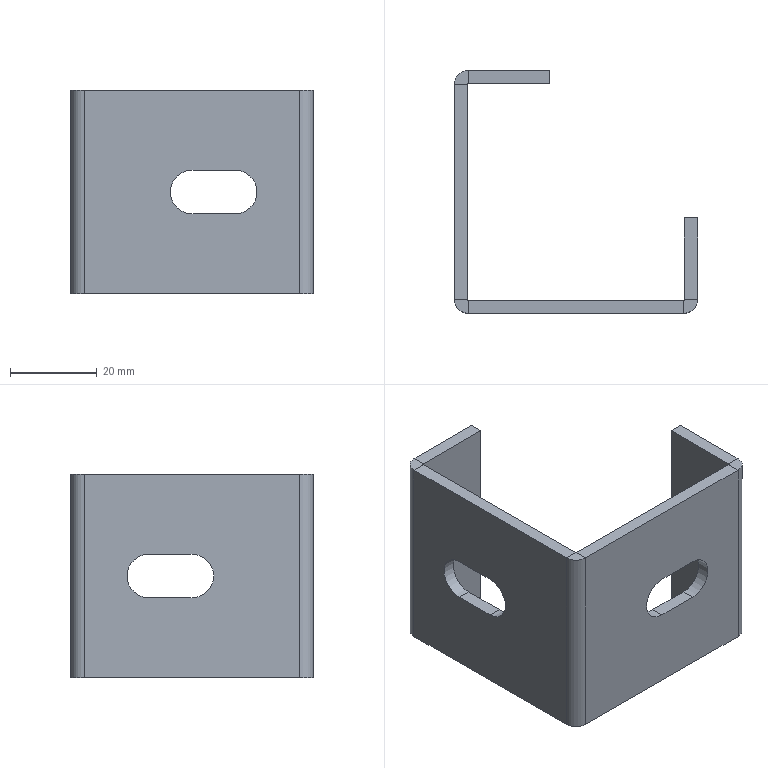Part | SolidWorks | features ICE 3, FlatPattern 1, SMBaseFlange 1, SheetMetal 1 | 1 solid | 39 faces | box 56 x 56 x 47 mm | volume 19347 mm3 | plane 28 | cylinder 11 | commonest cylinder face diameters 10 x5 0.4 x3 6.4 x3
STEP:
#1=CARTESIAN_POINT('',(3.,23.,0.));
#2=VERTEX_POINT('',#1);
#3=CARTESIAN_POINT('',(3.,28.,5.));
#4=VERTEX_POINT('',#3);
#5=CARTESIAN_POINT('',(3.,28.,0.));
#6=DIRECTION('',(-1.,0.,0.));
#7=DIRECTION('',(0.,-1.,0.));
#8=AXIS2_PLACEMENT_3D('',#5,#6,#7);
#9=CIRCLE('',#8,5.);
#10=EDGE_CURVE('',#2,#4,#9,.T.);
#11=ORIENTED_EDGE('',*,*,#10,.F.);
#12=CARTESIAN_POINT('',(0.,23.,0.));
#13=VERTEX_POINT('',#12);
#14=CARTESIAN_POINT('',(10.,23.,0.));
#15=DIRECTION('',(-1.,0.,0.));
#16=VECTOR('',#15,1000.);
#17=LINE('',#14,#16);
#18=EDGE_CURVE('',#2,#13,#17,.T.);
#19=ORIENTED_EDGE('',*,*,#18,.T.);
#20=CARTESIAN_POINT('',(0.,28.,5.));
#21=VERTEX_POINT('',#20);
#22=CARTESIAN_POINT('',(0.,28.,0.));
#23=DIRECTION('',(-1.,0.,0.));
#24=DIRECTION('',(0.,-1.,0.));
#25=AXIS2_PLACEMENT_3D('',#22,#23,#24);
#26=CIRCLE('',#25,5.);
#27=EDGE_CURVE('',#13,#21,#26,.T.);
#28=ORIENTED_EDGE('',*,*,#27,.T.);
#29=CARTESIAN_POINT('',(10.,28.,5.));
#30=DIRECTION('',(-1.,0.,0.));
#31=VECTOR('',#30,1000.);
#32=LINE('',#29,#31);
#33=EDGE_CURVE('',#4,#21,#32,.T.);
#34=ORIENTED_EDGE('',*,*,#33,.F.);
#35=EDGE_LOOP('',(#11,#19,#28,#34));
#36=FACE_OUTER_BOUND('',#35,.T.);
#37=CARTESIAN_POINT('',(10.,28.,0.));
#38=DIRECTION('',(-1.,0.,0.));
#39=DIRECTION('',(0.,-1.,0.));
#40=AXIS2_PLACEMENT_3D('',#37,#38,#39);
#41=CYLINDRICAL_SURFACE('',#40,5.);
#42=ADVANCED_FACE('',(#36),#41,.F.);
#43=CARTESIAN_POINT('',(52.8,0.,23.5));
#44=VERTEX_POINT('',#43);
#45=CARTESIAN_POINT('',(52.8,3.,23.5));
#46=VERTEX_POINT('',#45);
#47=CARTESIAN_POINT('',(52.8,0.,23.5));
#48=DIRECTION('',(0.,1.,0.));
#49=VECTOR('',#48,1000.);
#50=LINE('',#47,#49);
#51=EDGE_CURVE('',#44,#46,#50,.T.);
#52=ORIENTED_EDGE('',*,*,#51,.F.);
#53=CARTESIAN_POINT('',(56.,3.2,23.5));
#54=VERTEX_POINT('',#53);
#55=CARTESIAN_POINT('',(52.8,3.2,23.5));
#56=DIRECTION('',(0.,0.,-1.));
#57=DIRECTION('',(1.,0.,0.));
#58=AXIS2_PLACEMENT_3D('',#55,#56,#57);
#59=CIRCLE('',#58,3.2);
#60=EDGE_CURVE('',#54,#44,#59,.T.);
#61=ORIENTED_EDGE('',*,*,#60,.F.);
#62=CARTESIAN_POINT('',(53.,3.2,23.5));
#63=VERTEX_POINT('',#62);
#64=CARTESIAN_POINT('',(53.,3.2,23.5));
#65=DIRECTION('',(1.,0.,0.));
#66=VECTOR('',#65,1000.);
#67=LINE('',#64,#66);
#68=EDGE_CURVE('',#63,#54,#67,.T.);
#69=ORIENTED_EDGE('',*,*,#68,.F.);
#70=CARTESIAN_POINT('',(52.8,3.2,23.5));
#71=DIRECTION('',(0.,0.,-1.));
#72=DIRECTION('',(1.,0.,0.));
#73=AXIS2_PLACEMENT_3D('',#70,#71,#72);
#74=CIRCLE('',#73,0.2);
#75=EDGE_CURVE('',#63,#46,#74,.T.);
#76=ORIENTED_EDGE('',*,*,#75,.T.);
#77=EDGE_LOOP('',(#52,#61,#69,#76));
#78=FACE_OUTER_BOUND('',#77,.T.);
#79=CARTESIAN_POINT('',(52.8,0.,23.5));
#80=DIRECTION('',(0.,0.,1.));
#81=DIRECTION('',(1.,0.,0.));
#82=AXIS2_PLACEMENT_3D('',#79,#80,#81);
#83=PLANE('',#82);
#84=ADVANCED_FACE('',(#78),#83,.T.);
#85=CARTESIAN_POINT('',(3.2,0.,23.5));
#86=VERTEX_POINT('',#85);
#87=CARTESIAN_POINT('',(0.,0.,23.5));
#88=DIRECTION('',(-1.,0.,0.));
#89=VECTOR('',#88,1000.);
#90=LINE('',#87,#89);
#91=EDGE_CURVE('',#44,#86,#90,.T.);
#92=ORIENTED_EDGE('',*,*,#91,.F.);
#93=ORIENTED_EDGE('',*,*,#51,.T.);
#94=CARTESIAN_POINT('',(3.2,3.,23.5));
#95=VERTEX_POINT('',#94);
#96=CARTESIAN_POINT('',(0.,3.,23.5));
#97=DIRECTION('',(-1.,0.,0.));
#98=VECTOR('',#97,1000.);
#99=LINE('',#96,#98);
#100=EDGE_CURVE('',#46,#95,#99,.T.);
#101=ORIENTED_EDGE('',*,*,#100,.T.);
#102=CARTESIAN_POINT('',(3.2,3.,23.5));
#103=DIRECTION('',(0.,-1.,0.));
#104=VECTOR('',#103,1000.);
#105=LINE('',#102,#104);
#106=EDGE_CURVE('',#95,#86,#105,.T.);
#107=ORIENTED_EDGE('',*,*,#106,.T.);
#108=EDGE_LOOP('',(#92,#93,#101,#107));
#109=FACE_OUTER_BOUND('',#108,.T.);
#110=CARTESIAN_POINT('',(53.,3.2,23.5));
#111=DIRECTION('',(0.,0.,1.));
#112=DIRECTION('',(1.,0.,0.));
#113=AXIS2_PLACEMENT_3D('',#110,#111,#112);
#114=PLANE('',#113);
#115=ADVANCED_FACE('',(#109),#114,.T.);
#116=CARTESIAN_POINT('',(56.,3.2,-23.5));
#117=VERTEX_POINT('',#116);
#118=CARTESIAN_POINT('',(53.,3.2,-23.5));
#119=VERTEX_POINT('',#118);
#120=CARTESIAN_POINT('',(56.,3.2,-23.5));
#121=DIRECTION('',(-1.,0.,0.));
#122=VECTOR('',#121,1000.);
#123=LINE('',#120,#122);
#124=EDGE_CURVE('',#117,#119,#123,.T.);
#125=ORIENTED_EDGE('',*,*,#124,.F.);
#126=CARTESIAN_POINT('',(52.8,0.,-23.5));
#127=VERTEX_POINT('',#126);
#128=CARTESIAN_POINT('',(52.8,3.2,-23.5));
#129=DIRECTION('',(0.,0.,-1.));
#130=DIRECTION('',(1.,0.,0.));
#131=AXIS2_PLACEMENT_3D('',#128,#129,#130);
#132=CIRCLE('',#131,3.2);
#133=EDGE_CURVE('',#117,#127,#132,.T.);
#134=ORIENTED_EDGE('',*,*,#133,.T.);
#135=CARTESIAN_POINT('',(52.8,3.,-23.5));
#136=VERTEX_POINT('',#135);
#137=CARTESIAN_POINT('',(52.8,3.,-23.5));
#138=DIRECTION('',(0.,-1.,0.));
#139=VECTOR('',#138,1000.);
#140=LINE('',#137,#139);
#141=EDGE_CURVE('',#136,#127,#140,.T.);
#142=ORIENTED_EDGE('',*,*,#141,.F.);
#143=CARTESIAN_POINT('',(52.8,3.2,-23.5));
#144=DIRECTION('',(0.,0.,-1.));
#145=DIRECTION('',(1.,0.,0.));
#146=AXIS2_PLACEMENT_3D('',#143,#144,#145);
#147=CIRCLE('',#146,0.2);
#148=EDGE_CURVE('',#119,#136,#147,.T.);
#149=ORIENTED_EDGE('',*,*,#148,.F.);
#150=EDGE_LOOP('',(#125,#134,#142,#149));
#151=FACE_OUTER_BOUND('',#150,.T.);
#152=CARTESIAN_POINT('',(56.,3.2,-23.5));
#153=DIRECTION('',(0.,0.,-1.));
#154=DIRECTION('',(-1.,0.,0.));
#155=AXIS2_PLACEMENT_3D('',#152,#153,#154);
#156=PLANE('',#155);
#157=ADVANCED_FACE('',(#151),#156,.T.);
#158=CARTESIAN_POINT('',(56.,22.,-23.5));
#159=VERTEX_POINT('',#158);
#160=CARTESIAN_POINT('',(56.,0.,-23.5));
#161=DIRECTION('',(0.,-1.,0.));
#162=VECTOR('',#161,1000.);
#163=LINE('',#160,#162);
#164=EDGE_CURVE('',#159,#117,#163,.T.);
#165=ORIENTED_EDGE('',*,*,#164,.T.);
#166=ORIENTED_EDGE('',*,*,#124,.T.);
#167=CARTESIAN_POINT('',(53.,22.,-23.5));
#168=VERTEX_POINT('',#167);
#169=CARTESIAN_POINT('',(53.,0.,-23.5));
#170=DIRECTION('',(0.,-1.,0.));
#171=VECTOR('',#170,1000.);
#172=LINE('',#169,#171);
#173=EDGE_CURVE('',#168,#119,#172,.T.);
#174=ORIENTED_EDGE('',*,*,#173,.F.);
#175=CARTESIAN_POINT('',(53.,22.,-23.5));
#176=DIRECTION('',(1.,0.,0.));
#177=VECTOR('',#176,1000.);
#178=LINE('',#175,#177);
#179=EDGE_CURVE('',#168,#159,#178,.T.);
#180=ORIENTED_EDGE('',*,*,#179,.T.);
#181=EDGE_LOOP('',(#165,#166,#174,#180));
#182=FACE_OUTER_BOUND('',#181,.T.);
#183=CARTESIAN_POINT('',(52.8,3.,-23.5));
#184=DIRECTION('',(0.,0.,-1.));
#185=DIRECTION('',(-1.,0.,0.));
#186=AXIS2_PLACEMENT_3D('',#183,#184,#185);
#187=PLANE('',#186);
#188=ADVANCED_FACE('',(#182),#187,.T.);
#189=CARTESIAN_POINT('',(0.,3.2,23.5));
#190=VERTEX_POINT('',#189);
#191=CARTESIAN_POINT('',(3.,3.2,23.5));
#192=VERTEX_POINT('',#191);
#193=CARTESIAN_POINT('',(0.,3.2,23.5));
#194=DIRECTION('',(1.,0.,0.));
#195=VECTOR('',#194,1000.);
#196=LINE('',#193,#195);
#197=EDGE_CURVE('',#190,#192,#196,.T.);
#198=ORIENTED_EDGE('',*,*,#197,.F.);
#199=CARTESIAN_POINT('',(3.2,3.2,23.5));
#200=DIRECTION('',(0.,0.,-1.));
#201=DIRECTION('',(1.,0.,0.));
#202=AXIS2_PLACEMENT_3D('',#199,#200,#201);
#203=CIRCLE('',#202,3.2);
#204=EDGE_CURVE('',#86,#190,#203,.T.);
#205=ORIENTED_EDGE('',*,*,#204,.F.);
#206=ORIENTED_EDGE('',*,*,#106,.F.);
#207=CARTESIAN_POINT('',(3.2,3.2,23.5));
#208=DIRECTION('',(0.,0.,-1.));
#209=DIRECTION('',(1.,0.,0.));
#210=AXIS2_PLACEMENT_3D('',#207,#208,#209);
#211=CIRCLE('',#210,0.2);
#212=EDGE_CURVE('',#95,#192,#211,.T.);
#213=ORIENTED_EDGE('',*,*,#212,.T.);
#214=EDGE_LOOP('',(#198,#205,#206,#213));
#215=FACE_OUTER_BOUND('',#214,.T.);
#216=CARTESIAN_POINT('',(0.,3.2,23.5));
#217=DIRECTION('',(0.,0.,1.));
#218=DIRECTION('',(1.,0.,0.));
#219=AXIS2_PLACEMENT_3D('',#216,#217,#218);
#220=PLANE('',#219);
#221=ADVANCED_FACE('',(#215),#220,.T.);
#222=CARTESIAN_POINT('',(0.,52.8,23.5));
#223=VERTEX_POINT('',#222);
#224=CARTESIAN_POINT('',(0.,56.,23.5));
#225=DIRECTION('',(0.,1.,0.));
#226=VECTOR('',#225,1000.);
#227=LINE('',#224,#226);
#228=EDGE_CURVE('',#190,#223,#227,.T.);
#229=ORIENTED_EDGE('',*,*,#228,.F.);
#230=ORIENTED_EDGE('',*,*,#197,.T.);
#231=CARTESIAN_POINT('',(3.,52.8,23.5));
#232=VERTEX_POINT('',#231);
#233=CARTESIAN_POINT('',(3.,56.,23.5));
#234=DIRECTION('',(0.,1.,0.));
#235=VECTOR('',#234,1000.);
#236=LINE('',#233,#235);
#237=EDGE_CURVE('',#192,#232,#236,.T.);
#238=ORIENTED_EDGE('',*,*,#237,.T.);
#239=CARTESIAN_POINT('',(3.,52.8,23.5));
#240=DIRECTION('',(-1.,0.,0.));
#241=VECTOR('',#240,1000.);
#242=LINE('',#239,#241);
#243=EDGE_CURVE('',#232,#223,#242,.T.);
#244=ORIENTED_EDGE('',*,*,#243,.T.);
#245=EDGE_LOOP('',(#229,#230,#238,#244));
#246=FACE_OUTER_BOUND('',#245,.T.);
#247=CARTESIAN_POINT('',(3.2,3.,23.5));
#248=DIRECTION('',(0.,0.,1.));
#249=DIRECTION('',(1.,0.,0.));
#250=AXIS2_PLACEMENT_3D('',#247,#248,#249);
#251=PLANE('',#250);
#252=ADVANCED_FACE('',(#246),#251,.T.);
#253=CARTESIAN_POINT('',(3.2,0.,-23.5));
#254=VERTEX_POINT('',#253);
#255=CARTESIAN_POINT('',(3.2,3.,-23.5));
#256=VERTEX_POINT('',#255);
#257=CARTESIAN_POINT('',(3.2,0.,-23.5));
#258=DIRECTION('',(0.,1.,0.));
#259=VECTOR('',#258,1000.);
#260=LINE('',#257,#259);
#261=EDGE_CURVE('',#254,#256,#260,.T.);
#262=ORIENTED_EDGE('',*,*,#261,.F.);
#263=CARTESIAN_POINT('',(0.,3.2,-23.5));
#264=VERTEX_POINT('',#263);
#265=CARTESIAN_POINT('',(3.2,3.2,-23.5));
#266=DIRECTION('',(0.,0.,-1.));
#267=DIRECTION('',(1.,0.,0.));
#268=AXIS2_PLACEMENT_3D('',#265,#266,#267);
#269=CIRCLE('',#268,3.2);
#270=EDGE_CURVE('',#254,#264,#269,.T.);
#271=ORIENTED_EDGE('',*,*,#270,.T.);
#272=CARTESIAN_POINT('',(3.,3.2,-23.5));
#273=VERTEX_POINT('',#272);
#274=CARTESIAN_POINT('',(3.,3.2,-23.5));
#275=DIRECTION('',(-1.,0.,0.));
#276=VECTOR('',#275,1000.);
#277=LINE('',#274,#276);
#278=EDGE_CURVE('',#273,#264,#277,.T.);
#279=ORIENTED_EDGE('',*,*,#278,.F.);
#280=CARTESIAN_POINT('',(3.2,3.2,-23.5));
#281=DIRECTION('',(0.,0.,-1.));
#282=DIRECTION('',(1.,0.,0.));
#283=AXIS2_PLACEMENT_3D('',#280,#281,#282);
#284=CIRCLE('',#283,0.2);
#285=EDGE_CURVE('',#256,#273,#284,.T.);
#286=ORIENTED_EDGE('',*,*,#285,.F.);
#287=EDGE_LOOP('',(#262,#271,#279,#286));
#288=FACE_OUTER_BOUND('',#287,.T.);
#289=CARTESIAN_POINT('',(3.2,0.,-23.5));
#290=DIRECTION('',(0.,0.,-1.));
#291=DIRECTION('',(-1.,0.,0.));
#292=AXIS2_PLACEMENT_3D('',#289,#290,#291);
#293=PLANE('',#292);
#294=ADVANCED_FACE('',(#288),#293,.T.);
#295=CARTESIAN_POINT('',(0.,0.,-23.5));
#296=DIRECTION('',(-1.,0.,0.));
#297=VECTOR('',#296,1000.);
#298=LINE('',#295,#297);
#299=EDGE_CURVE('',#127,#254,#298,.T.);
#300=ORIENTED_EDGE('',*,*,#299,.T.);
#301=ORIENTED_EDGE('',*,*,#261,.T.);
#302=CARTESIAN_POINT('',(0.,3.,-23.5));
#303=DIRECTION('',(-1.,0.,0.));
#304=VECTOR('',#303,1000.);
#305=LINE('',#302,#304);
#306=EDGE_CURVE('',#136,#256,#305,.T.);
#307=ORIENTED_EDGE('',*,*,#306,.F.);
#308=ORIENTED_EDGE('',*,*,#141,.T.);
#309=EDGE_LOOP('',(#300,#301,#307,#308));
#310=FACE_OUTER_BOUND('',#309,.T.);
#311=CARTESIAN_POINT('',(3.,3.2,-23.5));
#312=DIRECTION('',(0.,0.,-1.));
#313=DIRECTION('',(-1.,0.,0.));
#314=AXIS2_PLACEMENT_3D('',#311,#312,#313);
#315=PLANE('',#314);
#316=ADVANCED_FACE('',(#310),#315,.T.);
#317=CARTESIAN_POINT('',(3.2,56.,23.5));
#318=VERTEX_POINT('',#317);
#319=CARTESIAN_POINT('',(3.2,53.,23.5));
#320=VERTEX_POINT('',#319);
#321=CARTESIAN_POINT('',(3.2,56.,23.5));
#322=DIRECTION('',(0.,-1.,0.));
#323=VECTOR('',#322,1000.);
#324=LINE('',#321,#323);
#325=EDGE_CURVE('',#318,#320,#324,.T.);
#326=ORIENTED_EDGE('',*,*,#325,.F.);
#327=CARTESIAN_POINT('',(3.2,52.8,23.5));
#328=DIRECTION('',(0.,0.,-1.));
#329=DIRECTION('',(1.,0.,0.));
#330=AXIS2_PLACEMENT_3D('',#327,#328,#329);
#331=CIRCLE('',#330,3.2);
#332=EDGE_CURVE('',#223,#318,#331,.T.);
#333=ORIENTED_EDGE('',*,*,#332,.F.);
#334=ORIENTED_EDGE('',*,*,#243,.F.);
#335=CARTESIAN_POINT('',(3.2,52.8,23.5));
#336=DIRECTION('',(0.,0.,-1.));
#337=DIRECTION('',(1.,0.,0.));
#338=AXIS2_PLACEMENT_3D('',#335,#336,#337);
#339=CIRCLE('',#338,0.2);
#340=EDGE_CURVE('',#232,#320,#339,.T.);
#341=ORIENTED_EDGE('',*,*,#340,.T.);
#342=EDGE_LOOP('',(#326,#333,#334,#341));
#343=FACE_OUTER_BOUND('',#342,.T.);
#344=CARTESIAN_POINT('',(3.2,56.,23.5));
#345=DIRECTION('',(0.,0.,1.));
#346=DIRECTION('',(1.,0.,0.));
#347=AXIS2_PLACEMENT_3D('',#344,#345,#346);
#348=PLANE('',#347);
#349=ADVANCED_FACE('',(#343),#348,.T.);
#350=CARTESIAN_POINT('',(22.,56.,23.5));
#351=VERTEX_POINT('',#350);
#352=CARTESIAN_POINT('',(0.,56.,23.5));
#353=DIRECTION('',(1.,0.,0.));
#354=VECTOR('',#353,1000.);
#355=LINE('',#352,#354);
#356=EDGE_CURVE('',#318,#351,#355,.T.);
#357=ORIENTED_EDGE('',*,*,#356,.F.);
#358=ORIENTED_EDGE('',*,*,#325,.T.);
#359=CARTESIAN_POINT('',(22.,53.,23.5));
#360=VERTEX_POINT('',#359);
#361=CARTESIAN_POINT('',(0.,53.,23.5));
#362=DIRECTION('',(1.,0.,0.));
#363=VECTOR('',#362,1000.);
#364=LINE('',#361,#363);
#365=EDGE_CURVE('',#320,#360,#364,.T.);
#366=ORIENTED_EDGE('',*,*,#365,.T.);
#367=CARTESIAN_POINT('',(22.,56.,23.5));
#368=DIRECTION('',(0.,-1.,0.));
#369=VECTOR('',#368,1000.);
#370=LINE('',#367,#369);
#371=EDGE_CURVE('',#351,#360,#370,.T.);
#372=ORIENTED_EDGE('',*,*,#371,.F.);
#373=EDGE_LOOP('',(#357,#358,#366,#372));
#374=FACE_OUTER_BOUND('',#373,.T.);
#375=CARTESIAN_POINT('',(3.,52.8,23.5));
#376=DIRECTION('',(0.,0.,1.));
#377=DIRECTION('',(1.,0.,0.));
#378=AXIS2_PLACEMENT_3D('',#375,#376,#377);
#379=PLANE('',#378);
#380=ADVANCED_FACE('',(#374),#379,.T.);
#381=CARTESIAN_POINT('',(0.,52.8,-23.5));
#382=VERTEX_POINT('',#381);
#383=CARTESIAN_POINT('',(3.,52.8,-23.5));
#384=VERTEX_POINT('',#383);
#385=CARTESIAN_POINT('',(0.,52.8,-23.5));
#386=DIRECTION('',(1.,0.,0.));
#387=VECTOR('',#386,1000.);
#388=LINE('',#385,#387);
#389=EDGE_CURVE('',#382,#384,#388,.T.);
#390=ORIENTED_EDGE('',*,*,#389,.F.);
#391=CARTESIAN_POINT('',(3.2,56.,-23.5));
#392=VERTEX_POINT('',#391);
#393=CARTESIAN_POINT('',(3.2,52.8,-23.5));
#394=DIRECTION('',(0.,0.,-1.));
#395=DIRECTION('',(1.,0.,0.));
#396=AXIS2_PLACEMENT_3D('',#393,#394,#395);
#397=CIRCLE('',#396,3.2);
#398=EDGE_CURVE('',#382,#392,#397,.T.);
#399=ORIENTED_EDGE('',*,*,#398,.T.);
#400=CARTESIAN_POINT('',(3.2,53.,-23.5));
#401=VERTEX_POINT('',#400);
#402=CARTESIAN_POINT('',(3.2,53.,-23.5));
#403=DIRECTION('',(0.,1.,0.));
#404=VECTOR('',#403,1000.);
#405=LINE('',#402,#404);
#406=EDGE_CURVE('',#401,#392,#405,.T.);
#407=ORIENTED_EDGE('',*,*,#406,.F.);
#408=CARTESIAN_POINT('',(3.2,52.8,-23.5));
#409=DIRECTION('',(0.,0.,-1.));
#410=DIRECTION('',(1.,0.,0.));
#411=AXIS2_PLACEMENT_3D('',#408,#409,#410);
#412=CIRCLE('',#411,0.2);
#413=EDGE_CURVE('',#384,#401,#412,.T.);
#414=ORIENTED_EDGE('',*,*,#413,.F.);
#415=EDGE_LOOP('',(#390,#399,#407,#414));
#416=FACE_OUTER_BOUND('',#415,.T.);
#417=CARTESIAN_POINT('',(0.,52.8,-23.5));
#418=DIRECTION('',(0.,0.,-1.));
#419=DIRECTION('',(-1.,0.,0.));
#420=AXIS2_PLACEMENT_3D('',#417,#418,#419);
#421=PLANE('',#420);
#422=ADVANCED_FACE('',(#416),#421,.T.);
#423=CARTESIAN_POINT('',(0.,56.,-23.5));
#424=DIRECTION('',(0.,1.,0.));
#425=VECTOR('',#424,1000.);
#426=LINE('',#423,#425);
#427=EDGE_CURVE('',#264,#382,#426,.T.);
#428=ORIENTED_EDGE('',*,*,#427,.T.);
#429=ORIENTED_EDGE('',*,*,#389,.T.);
#430=CARTESIAN_POINT('',(3.,56.,-23.5));
#431=DIRECTION('',(0.,1.,0.));
#432=VECTOR('',#431,1000.);
#433=LINE('',#430,#432);
#434=EDGE_CURVE('',#273,#384,#433,.T.);
#435=ORIENTED_EDGE('',*,*,#434,.F.);
#436=ORIENTED_EDGE('',*,*,#278,.T.);
#437=EDGE_LOOP('',(#428,#429,#435,#436));
#438=FACE_OUTER_BOUND('',#437,.T.);
#439=CARTESIAN_POINT('',(3.2,53.,-23.5));
#440=DIRECTION('',(0.,0.,-1.));
#441=DIRECTION('',(-1.,0.,0.));
#442=AXIS2_PLACEMENT_3D('',#439,#440,#441);
#443=PLANE('',#442);
#444=ADVANCED_FACE('',(#438),#443,.T.);
#445=CARTESIAN_POINT('',(22.,53.,-23.5));
#446=VERTEX_POINT('',#445);
#447=CARTESIAN_POINT('',(0.,53.,-23.5));
#448=DIRECTION('',(1.,0.,0.));
#449=VECTOR('',#448,1000.);
#450=LINE('',#447,#449);
#451=EDGE_CURVE('',#401,#446,#450,.T.);
#452=ORIENTED_EDGE('',*,*,#451,.T.);
#453=CARTESIAN_POINT('',(22.,53.,23.5));
#454=DIRECTION('',(0.,0.,-1.));
#455=VECTOR('',#454,1000.);
#456=LINE('',#453,#455);
#457=EDGE_CURVE('',#360,#446,#456,.T.);
#458=ORIENTED_EDGE('',*,*,#457,.F.);
#459=ORIENTED_EDGE('',*,*,#365,.F.);
#460=CARTESIAN_POINT('',(3.2,53.,23.5));
#461=DIRECTION('',(0.,0.,-1.));
#462=VECTOR('',#461,1000.);
#463=LINE('',#460,#462);
#464=EDGE_CURVE('',#320,#401,#463,.T.);
#465=ORIENTED_EDGE('',*,*,#464,.T.);
#466=EDGE_LOOP('',(#452,#458,#459,#465));
#467=FACE_OUTER_BOUND('',#466,.T.);
#468=CARTESIAN_POINT('',(0.,53.,23.5));
#469=DIRECTION('',(0.,1.,0.));
#470=DIRECTION('',(0.,0.,1.));
#471=AXIS2_PLACEMENT_3D('',#468,#469,#470);
#472=PLANE('',#471);
#473=ADVANCED_FACE('',(#467),#472,.F.);
#474=CARTESIAN_POINT('',(22.,56.,-23.5));
#475=VERTEX_POINT('',#474);
#476=CARTESIAN_POINT('',(22.,56.,-23.5));
#477=DIRECTION('',(0.,-1.,0.));
#478=VECTOR('',#477,1000.);
#479=LINE('',#476,#478);
#480=EDGE_CURVE('',#475,#446,#479,.T.);
#481=ORIENTED_EDGE('',*,*,#480,.F.);
#482=CARTESIAN_POINT('',(22.,56.,23.5));
#483=DIRECTION('',(0.,0.,-1.));
#484=VECTOR('',#483,1000.);
#485=LINE('',#482,#484);
#486=EDGE_CURVE('',#351,#475,#485,.T.);
#487=ORIENTED_EDGE('',*,*,#486,.F.);
#488=ORIENTED_EDGE('',*,*,#371,.T.);
#489=ORIENTED_EDGE('',*,*,#457,.T.);
#490=EDGE_LOOP('',(#481,#487,#488,#489));
#491=FACE_OUTER_BOUND('',#490,.T.);
#492=CARTESIAN_POINT('',(22.,56.,23.5));
#493=DIRECTION('',(1.,0.,0.));
#494=DIRECTION('',(0.,0.,-1.));
#495=AXIS2_PLACEMENT_3D('',#492,#493,#494);
#496=PLANE('',#495);
#497=ADVANCED_FACE('',(#491),#496,.T.);
#498=CARTESIAN_POINT('',(0.,56.,-23.5));
#499=DIRECTION('',(1.,0.,0.));
#500=VECTOR('',#499,1000.);
#501=LINE('',#498,#500);
#502=EDGE_CURVE('',#392,#475,#501,.T.);
#503=ORIENTED_EDGE('',*,*,#502,.F.);
#504=CARTESIAN_POINT('',(3.2,56.,23.5));
#505=DIRECTION('',(0.,0.,-1.));
#506=VECTOR('',#505,1000.);
#507=LINE('',#504,#506);
#508=EDGE_CURVE('',#318,#392,#507,.T.);
#509=ORIENTED_EDGE('',*,*,#508,.F.);
#510=ORIENTED_EDGE('',*,*,#356,.T.);
#511=ORIENTED_EDGE('',*,*,#486,.T.);
#512=EDGE_LOOP('',(#503,#509,#510,#511));
#513=FACE_OUTER_BOUND('',#512,.T.);
#514=CARTESIAN_POINT('',(0.,56.,23.5));
#515=DIRECTION('',(0.,1.,0.));
#516=DIRECTION('',(0.,0.,1.));
#517=AXIS2_PLACEMENT_3D('',#514,#515,#516);
#518=PLANE('',#517);
#519=ADVANCED_FACE('',(#513),#518,.T.);
#520=ORIENTED_EDGE('',*,*,#398,.F.);
#521=CARTESIAN_POINT('',(0.,52.8,23.5));
#522=DIRECTION('',(0.,0.,-1.));
#523=VECTOR('',#522,1000.);
#524=LINE('',#521,#523);
#525=EDGE_CURVE('',#223,#382,#524,.T.);
#526=ORIENTED_EDGE('',*,*,#525,.F.);
#527=ORIENTED_EDGE('',*,*,#332,.T.);
#528=ORIENTED_EDGE('',*,*,#508,.T.);
#529=EDGE_LOOP('',(#520,#526,#527,#528));
#530=FACE_OUTER_BOUND('',#529,.T.);
#531=CARTESIAN_POINT('',(3.2,52.8,23.5));
#532=DIRECTION('',(0.,0.,-1.));
#533=DIRECTION('',(-1.,0.,0.));
#534=AXIS2_PLACEMENT_3D('',#531,#532,#533);
#535=CYLINDRICAL_SURFACE('',#534,3.2);
#536=ADVANCED_FACE('',(#530),#535,.T.);
#537=CARTESIAN_POINT('',(0.,28.,-5.));
#538=VERTEX_POINT('',#537);
#539=CARTESIAN_POINT('',(0.,28.,0.));
#540=DIRECTION('',(-1.,0.,0.));
#541=DIRECTION('',(0.,-1.,0.));
#542=AXIS2_PLACEMENT_3D('',#539,#540,#541);
#543=CIRCLE('',#542,5.);
#544=EDGE_CURVE('',#538,#13,#543,.T.);
#545=ORIENTED_EDGE('',*,*,#544,.F.);
#546=CARTESIAN_POINT('',(0.,38.,-5.));
#547=VERTEX_POINT('',#546);
#548=CARTESIAN_POINT('',(0.,28.,-5.));
#549=DIRECTION('',(0.,-1.,0.));
#550=VECTOR('',#549,1000.);
#551=LINE('',#548,#550);
#552=EDGE_CURVE('',#547,#538,#551,.T.);
#553=ORIENTED_EDGE('',*,*,#552,.F.);
#554=CARTESIAN_POINT('',(0.,38.,5.));
#555=VERTEX_POINT('',#554);
#556=CARTESIAN_POINT('',(0.,38.,0.));
#557=DIRECTION('',(-1.,0.,0.));
#558=DIRECTION('',(0.,-1.,0.));
#559=AXIS2_PLACEMENT_3D('',#556,#557,#558);
#560=CIRCLE('',#559,5.);
#561=EDGE_CURVE('',#555,#547,#560,.T.);
#562=ORIENTED_EDGE('',*,*,#561,.F.);
#563=CARTESIAN_POINT('',(0.,28.,5.));
#564=DIRECTION('',(0.,1.,0.));
#565=VECTOR('',#564,1000.);
#566=LINE('',#563,#565);
#567=EDGE_CURVE('',#21,#555,#566,.T.);
#568=ORIENTED_EDGE('',*,*,#567,.F.);
#569=ORIENTED_EDGE('',*,*,#27,.F.);
#570=EDGE_LOOP('',(#545,#553,#562,#568,#569));
#571=FACE_BOUND('',#570,.T.);
#572=ORIENTED_EDGE('',*,*,#427,.F.);
#573=CARTESIAN_POINT('',(0.,3.2,23.5));
#574=DIRECTION('',(0.,0.,-1.));
#575=VECTOR('',#574,1000.);
#576=LINE('',#573,#575);
#577=EDGE_CURVE('',#190,#264,#576,.T.);
#578=ORIENTED_EDGE('',*,*,#577,.F.);
#579=ORIENTED_EDGE('',*,*,#228,.T.);
#580=ORIENTED_EDGE('',*,*,#525,.T.);
#581=EDGE_LOOP('',(#572,#578,#579,#580));
#582=FACE_OUTER_BOUND('',#581,.T.);
#583=CARTESIAN_POINT('',(0.,56.,23.5));
#584=DIRECTION('',(-1.,0.,0.));
#585=DIRECTION('',(0.,-1.,0.));
#586=AXIS2_PLACEMENT_3D('',#583,#584,#585);
#587=PLANE('',#586);
#588=ADVANCED_FACE('',(#571,#582),#587,.T.);
#589=ORIENTED_EDGE('',*,*,#270,.F.);
#590=CARTESIAN_POINT('',(3.2,0.,23.5));
#591=DIRECTION('',(0.,0.,-1.));
#592=VECTOR('',#591,1000.);
#593=LINE('',#590,#592);
#594=EDGE_CURVE('',#86,#254,#593,.T.);
#595=ORIENTED_EDGE('',*,*,#594,.F.);
#596=ORIENTED_EDGE('',*,*,#204,.T.);
#597=ORIENTED_EDGE('',*,*,#577,.T.);
#598=EDGE_LOOP('',(#589,#595,#596,#597));
#599=FACE_OUTER_BOUND('',#598,.T.);
#600=CARTESIAN_POINT('',(3.2,3.2,23.5));
#601=DIRECTION('',(0.,0.,-1.));
#602=DIRECTION('',(-1.,0.,0.));
#603=AXIS2_PLACEMENT_3D('',#600,#601,#602);
#604=CYLINDRICAL_SURFACE('',#603,3.2);
#605=ADVANCED_FACE('',(#599),#604,.T.);
#606=CARTESIAN_POINT('',(38.,0.,-5.));
#607=VERTEX_POINT('',#606);
#608=CARTESIAN_POINT('',(38.,0.,5.));
#609=VERTEX_POINT('',#608);
#610=CARTESIAN_POINT('',(38.,0.,0.));
#611=DIRECTION('',(0.,-1.,0.));
#612=DIRECTION('',(0.,0.,-1.));
#613=AXIS2_PLACEMENT_3D('',#610,#611,#612);
#614=CIRCLE('',#613,5.);
#615=EDGE_CURVE('',#607,#609,#614,.T.);
#616=ORIENTED_EDGE('',*,*,#615,.F.);
#617=CARTESIAN_POINT('',(28.,0.,-5.));
#618=VERTEX_POINT('',#617);
#619=CARTESIAN_POINT('',(38.,0.,-5.));
#620=DIRECTION('',(1.,0.,0.));
#621=VECTOR('',#620,1000.);
#622=LINE('',#619,#621);
#623=EDGE_CURVE('',#618,#607,#622,.T.);
#624=ORIENTED_EDGE('',*,*,#623,.F.);
#625=CARTESIAN_POINT('',(28.,0.,5.));
#626=VERTEX_POINT('',#625);
#627=CARTESIAN_POINT('',(28.,0.,0.));
#628=DIRECTION('',(0.,-1.,0.));
#629=DIRECTION('',(0.,0.,-1.));
#630=AXIS2_PLACEMENT_3D('',#627,#628,#629);
#631=CIRCLE('',#630,5.);
#632=EDGE_CURVE('',#626,#618,#631,.T.);
#633=ORIENTED_EDGE('',*,*,#632,.F.);
#634=CARTESIAN_POINT('',(38.,0.,5.));
#635=DIRECTION('',(-1.,0.,0.));
#636=VECTOR('',#635,1000.);
#637=LINE('',#634,#636);
#638=EDGE_CURVE('',#609,#626,#637,.T.);
#639=ORIENTED_EDGE('',*,*,#638,.F.);
#640=EDGE_LOOP('',(#616,#624,#633,#639));
#641=FACE_BOUND('',#640,.T.);
#642=ORIENTED_EDGE('',*,*,#299,.F.);
#643=CARTESIAN_POINT('',(52.8,0.,23.5));
#644=DIRECTION('',(0.,0.,-1.));
#645=VECTOR('',#644,1000.);
#646=LINE('',#643,#645);
#647=EDGE_CURVE('',#44,#127,#646,.T.);
#648=ORIENTED_EDGE('',*,*,#647,.F.);
#649=ORIENTED_EDGE('',*,*,#91,.T.);
#650=ORIENTED_EDGE('',*,*,#594,.T.);
#651=EDGE_LOOP('',(#642,#648,#649,#650));
#652=FACE_OUTER_BOUND('',#651,.T.);
#653=CARTESIAN_POINT('',(0.,0.,23.5));
#654=DIRECTION('',(0.,-1.,0.));
#655=DIRECTION('',(0.,0.,-1.));
#656=AXIS2_PLACEMENT_3D('',#653,#654,#655);
#657=PLANE('',#656);
#658=ADVANCED_FACE('',(#641,#652),#657,.T.);
#659=ORIENTED_EDGE('',*,*,#133,.F.);
#660=CARTESIAN_POINT('',(56.,3.2,23.5));
#661=DIRECTION('',(0.,0.,-1.));
#662=VECTOR('',#661,1000.);
#663=LINE('',#660,#662);
#664=EDGE_CURVE('',#54,#117,#663,.T.);
#665=ORIENTED_EDGE('',*,*,#664,.F.);
#666=ORIENTED_EDGE('',*,*,#60,.T.);
#667=ORIENTED_EDGE('',*,*,#647,.T.);
#668=EDGE_LOOP('',(#659,#665,#666,#667));
#669=FACE_OUTER_BOUND('',#668,.T.);
#670=CARTESIAN_POINT('',(52.8,3.2,23.5));
#671=DIRECTION('',(0.,0.,-1.));
#672=DIRECTION('',(-1.,0.,0.));
#673=AXIS2_PLACEMENT_3D('',#670,#671,#672);
#674=CYLINDRICAL_SURFACE('',#673,3.2);
#675=ADVANCED_FACE('',(#669),#674,.T.);
#676=ORIENTED_EDGE('',*,*,#164,.F.);
#677=CARTESIAN_POINT('',(56.,22.,23.5));
#678=VERTEX_POINT('',#677);
#679=CARTESIAN_POINT('',(56.,22.,23.5));
#680=DIRECTION('',(0.,0.,-1.));
#681=VECTOR('',#680,1000.);
#682=LINE('',#679,#681);
#683=EDGE_CURVE('',#678,#159,#682,.T.);
#684=ORIENTED_EDGE('',*,*,#683,.F.);
#685=CARTESIAN_POINT('',(56.,0.,23.5));
#686=DIRECTION('',(0.,-1.,0.));
#687=VECTOR('',#686,1000.);
#688=LINE('',#685,#687);
#689=EDGE_CURVE('',#678,#54,#688,.T.);
#690=ORIENTED_EDGE('',*,*,#689,.T.);
#691=ORIENTED_EDGE('',*,*,#664,.T.);
#692=EDGE_LOOP('',(#676,#684,#690,#691));
#693=FACE_OUTER_BOUND('',#692,.T.);
#694=CARTESIAN_POINT('',(56.,0.,23.5));
#695=DIRECTION('',(1.,0.,0.));
#696=DIRECTION('',(0.,0.,-1.));
#697=AXIS2_PLACEMENT_3D('',#694,#695,#696);
#698=PLANE('',#697);
#699=ADVANCED_FACE('',(#693),#698,.T.);
#700=ORIENTED_EDGE('',*,*,#179,.F.);
#701=CARTESIAN_POINT('',(53.,22.,23.5));
#702=VERTEX_POINT('',#701);
#703=CARTESIAN_POINT('',(53.,22.,23.5));
#704=DIRECTION('',(0.,0.,-1.));
#705=VECTOR('',#704,1000.);
#706=LINE('',#703,#705);
#707=EDGE_CURVE('',#702,#168,#706,.T.);
#708=ORIENTED_EDGE('',*,*,#707,.F.);
#709=CARTESIAN_POINT('',(53.,22.,23.5));
#710=DIRECTION('',(1.,0.,0.));
#711=VECTOR('',#710,1000.);
#712=LINE('',#709,#711);
#713=EDGE_CURVE('',#702,#678,#712,.T.);
#714=ORIENTED_EDGE('',*,*,#713,.T.);
#715=ORIENTED_EDGE('',*,*,#683,.T.);
#716=EDGE_LOOP('',(#700,#708,#714,#715));
#717=FACE_OUTER_BOUND('',#716,.T.);
#718=CARTESIAN_POINT('',(53.,22.,23.5));
#719=DIRECTION('',(0.,1.,0.));
#720=DIRECTION('',(0.,0.,1.));
#721=AXIS2_PLACEMENT_3D('',#718,#719,#720);
#722=PLANE('',#721);
#723=ADVANCED_FACE('',(#717),#722,.T.);
#724=ORIENTED_EDGE('',*,*,#173,.T.);
#725=CARTESIAN_POINT('',(53.,3.2,23.5));
#726=DIRECTION('',(0.,0.,-1.));
#727=VECTOR('',#726,1000.);
#728=LINE('',#725,#727);
#729=EDGE_CURVE('',#63,#119,#728,.T.);
#730=ORIENTED_EDGE('',*,*,#729,.F.);
#731=CARTESIAN_POINT('',(53.,0.,23.5));
#732=DIRECTION('',(0.,-1.,0.));
#733=VECTOR('',#732,1000.);
#734=LINE('',#731,#733);
#735=EDGE_CURVE('',#702,#63,#734,.T.);
#736=ORIENTED_EDGE('',*,*,#735,.F.);
#737=ORIENTED_EDGE('',*,*,#707,.T.);
#738=EDGE_LOOP('',(#724,#730,#736,#737));
#739=FACE_OUTER_BOUND('',#738,.T.);
#740=CARTESIAN_POINT('',(53.,0.,23.5));
#741=DIRECTION('',(1.,0.,0.));
#742=DIRECTION('',(0.,0.,-1.));
#743=AXIS2_PLACEMENT_3D('',#740,#741,#742);
#744=PLANE('',#743);
#745=ADVANCED_FACE('',(#739),#744,.F.);
#746=ORIENTED_EDGE('',*,*,#148,.T.);
#747=CARTESIAN_POINT('',(52.8,3.,23.5));
#748=DIRECTION('',(0.,0.,-1.));
#749=VECTOR('',#748,1000.);
#750=LINE('',#747,#749);
#751=EDGE_CURVE('',#46,#136,#750,.T.);
#752=ORIENTED_EDGE('',*,*,#751,.F.);
#753=ORIENTED_EDGE('',*,*,#75,.F.);
#754=ORIENTED_EDGE('',*,*,#729,.T.);
#755=EDGE_LOOP('',(#746,#752,#753,#754));
#756=FACE_OUTER_BOUND('',#755,.T.);
#757=CARTESIAN_POINT('',(52.8,3.2,23.5));
#758=DIRECTION('',(0.,0.,-1.));
#759=DIRECTION('',(-1.,0.,0.));
#760=AXIS2_PLACEMENT_3D('',#757,#758,#759);
#761=CYLINDRICAL_SURFACE('',#760,0.2);
#762=ADVANCED_FACE('',(#756),#761,.F.);
#763=CARTESIAN_POINT('',(28.,3.,-5.));
#764=VERTEX_POINT('',#763);
#765=CARTESIAN_POINT('',(38.,3.,-5.));
#766=VERTEX_POINT('',#765);
#767=CARTESIAN_POINT('',(0.,3.,-5.));
#768=DIRECTION('',(1.,0.,0.));
#769=VECTOR('',#768,1000.);
#770=LINE('',#767,#769);
#771=EDGE_CURVE('',#764,#766,#770,.T.);
#772=ORIENTED_EDGE('',*,*,#771,.T.);
#773=CARTESIAN_POINT('',(38.,3.,5.));
#774=VERTEX_POINT('',#773);
#775=CARTESIAN_POINT('',(38.,3.,0.));
#776=DIRECTION('',(0.,-1.,0.));
#777=DIRECTION('',(0.,0.,-1.));
#778=AXIS2_PLACEMENT_3D('',#775,#776,#777);
#779=CIRCLE('',#778,5.);
#780=EDGE_CURVE('',#766,#774,#779,.T.);
#781=ORIENTED_EDGE('',*,*,#780,.T.);
#782=CARTESIAN_POINT('',(28.,3.,5.));
#783=VERTEX_POINT('',#782);
#784=CARTESIAN_POINT('',(0.,3.,5.));
#785=DIRECTION('',(-1.,0.,0.));
#786=VECTOR('',#785,1000.);
#787=LINE('',#784,#786);
#788=EDGE_CURVE('',#774,#783,#787,.T.);
#789=ORIENTED_EDGE('',*,*,#788,.T.);
#790=CARTESIAN_POINT('',(28.,3.,0.));
#791=DIRECTION('',(0.,-1.,0.));
#792=DIRECTION('',(0.,0.,-1.));
#793=AXIS2_PLACEMENT_3D('',#790,#791,#792);
#794=CIRCLE('',#793,5.);
#795=EDGE_CURVE('',#783,#764,#794,.T.);
#796=ORIENTED_EDGE('',*,*,#795,.T.);
#797=EDGE_LOOP('',(#772,#781,#789,#796));
#798=FACE_BOUND('',#797,.T.);
#799=ORIENTED_EDGE('',*,*,#306,.T.);
#800=CARTESIAN_POINT('',(3.2,3.,23.5));
#801=DIRECTION('',(0.,0.,-1.));
#802=VECTOR('',#801,1000.);
#803=LINE('',#800,#802);
#804=EDGE_CURVE('',#95,#256,#803,.T.);
#805=ORIENTED_EDGE('',*,*,#804,.F.);
#806=ORIENTED_EDGE('',*,*,#100,.F.);
#807=ORIENTED_EDGE('',*,*,#751,.T.);
#808=EDGE_LOOP('',(#799,#805,#806,#807));
#809=FACE_OUTER_BOUND('',#808,.T.);
#810=CARTESIAN_POINT('',(0.,3.,23.5));
#811=DIRECTION('',(0.,-1.,0.));
#812=DIRECTION('',(0.,0.,-1.));
#813=AXIS2_PLACEMENT_3D('',#810,#811,#812);
#814=PLANE('',#813);
#815=ADVANCED_FACE('',(#798,#809),#814,.F.);
#816=ORIENTED_EDGE('',*,*,#285,.T.);
#817=CARTESIAN_POINT('',(3.,3.2,23.5));
#818=DIRECTION('',(0.,0.,-1.));
#819=VECTOR('',#818,1000.);
#820=LINE('',#817,#819);
#821=EDGE_CURVE('',#192,#273,#820,.T.);
#822=ORIENTED_EDGE('',*,*,#821,.F.);
#823=ORIENTED_EDGE('',*,*,#212,.F.);
#824=ORIENTED_EDGE('',*,*,#804,.T.);
#825=EDGE_LOOP('',(#816,#822,#823,#824));
#826=FACE_OUTER_BOUND('',#825,.T.);
#827=CARTESIAN_POINT('',(3.2,3.2,23.5));
#828=DIRECTION('',(0.,0.,-1.));
#829=DIRECTION('',(-1.,0.,0.));
#830=AXIS2_PLACEMENT_3D('',#827,#828,#829);
#831=CYLINDRICAL_SURFACE('',#830,0.2);
#832=ADVANCED_FACE('',(#826),#831,.F.);
#833=CARTESIAN_POINT('',(3.,38.,-5.));
#834=VERTEX_POINT('',#833);
#835=CARTESIAN_POINT('',(3.,28.,-5.));
#836=VERTEX_POINT('',#835);
#837=CARTESIAN_POINT('',(3.,56.,-5.));
#838=DIRECTION('',(0.,-1.,0.));
#839=VECTOR('',#838,1000.);
#840=LINE('',#837,#839);
#841=EDGE_CURVE('',#834,#836,#840,.T.);
#842=ORIENTED_EDGE('',*,*,#841,.T.);
#843=CARTESIAN_POINT('',(3.,28.,0.));
#844=DIRECTION('',(-1.,0.,0.));
#845=DIRECTION('',(0.,-1.,0.));
#846=AXIS2_PLACEMENT_3D('',#843,#844,#845);
#847=CIRCLE('',#846,5.);
#848=EDGE_CURVE('',#836,#2,#847,.T.);
#849=ORIENTED_EDGE('',*,*,#848,.T.);
#850=ORIENTED_EDGE('',*,*,#10,.T.);
#851=CARTESIAN_POINT('',(3.,38.,5.));
#852=VERTEX_POINT('',#851);
#853=CARTESIAN_POINT('',(3.,56.,5.));
#854=DIRECTION('',(0.,1.,0.));
#855=VECTOR('',#854,1000.);
#856=LINE('',#853,#855);
#857=EDGE_CURVE('',#4,#852,#856,.T.);
#858=ORIENTED_EDGE('',*,*,#857,.T.);
#859=CARTESIAN_POINT('',(3.,38.,0.));
#860=DIRECTION('',(-1.,0.,0.));
#861=DIRECTION('',(0.,-1.,0.));
#862=AXIS2_PLACEMENT_3D('',#859,#860,#861);
#863=CIRCLE('',#862,5.);
#864=EDGE_CURVE('',#852,#834,#863,.T.);
#865=ORIENTED_EDGE('',*,*,#864,.T.);
#866=EDGE_LOOP('',(#842,#849,#850,#858,#865));
#867=FACE_BOUND('',#866,.T.);
#868=ORIENTED_EDGE('',*,*,#434,.T.);
#869=CARTESIAN_POINT('',(3.,52.8,23.5));
#870=DIRECTION('',(0.,0.,-1.));
#871=VECTOR('',#870,1000.);
#872=LINE('',#869,#871);
#873=EDGE_CURVE('',#232,#384,#872,.T.);
#874=ORIENTED_EDGE('',*,*,#873,.F.);
#875=ORIENTED_EDGE('',*,*,#237,.F.);
#876=ORIENTED_EDGE('',*,*,#821,.T.);
#877=EDGE_LOOP('',(#868,#874,#875,#876));
#878=FACE_OUTER_BOUND('',#877,.T.);
#879=CARTESIAN_POINT('',(3.,56.,23.5));
#880=DIRECTION('',(-1.,0.,0.));
#881=DIRECTION('',(0.,-1.,0.));
#882=AXIS2_PLACEMENT_3D('',#879,#880,#881);
#883=PLANE('',#882);
#884=ADVANCED_FACE('',(#867,#878),#883,.F.);
#885=ORIENTED_EDGE('',*,*,#413,.T.);
#886=ORIENTED_EDGE('',*,*,#464,.F.);
#887=ORIENTED_EDGE('',*,*,#340,.F.);
#888=ORIENTED_EDGE('',*,*,#873,.T.);
#889=EDGE_LOOP('',(#885,#886,#887,#888));
#890=FACE_OUTER_BOUND('',#889,.T.);
#891=CARTESIAN_POINT('',(3.2,52.8,23.5));
#892=DIRECTION('',(0.,0.,-1.));
#893=DIRECTION('',(-1.,0.,0.));
#894=AXIS2_PLACEMENT_3D('',#891,#892,#893);
#895=CYLINDRICAL_SURFACE('',#894,0.2);
#896=ADVANCED_FACE('',(#890),#895,.F.);
#897=ORIENTED_EDGE('',*,*,#735,.T.);
#898=ORIENTED_EDGE('',*,*,#68,.T.);
#899=ORIENTED_EDGE('',*,*,#689,.F.);
#900=ORIENTED_EDGE('',*,*,#713,.F.);
#901=EDGE_LOOP('',(#897,#898,#899,#900));
#902=FACE_OUTER_BOUND('',#901,.T.);
#903=CARTESIAN_POINT('',(3.2,52.8,23.5));
#904=DIRECTION('',(0.,0.,1.));
#905=DIRECTION('',(1.,0.,0.));
#906=AXIS2_PLACEMENT_3D('',#903,#904,#905);
#907=PLANE('',#906);
#908=ADVANCED_FACE('',(#902),#907,.T.);
#909=ORIENTED_EDGE('',*,*,#451,.F.);
#910=ORIENTED_EDGE('',*,*,#406,.T.);
#911=ORIENTED_EDGE('',*,*,#502,.T.);
#912=ORIENTED_EDGE('',*,*,#480,.T.);
#913=EDGE_LOOP('',(#909,#910,#911,#912));
#914=FACE_OUTER_BOUND('',#913,.T.);
#915=CARTESIAN_POINT('',(3.2,52.8,-23.5));
#916=DIRECTION('',(0.,0.,1.));
#917=DIRECTION('',(1.,0.,0.));
#918=AXIS2_PLACEMENT_3D('',#915,#916,#917);
#919=PLANE('',#918);
#920=ADVANCED_FACE('',(#914),#919,.F.);
#921=CARTESIAN_POINT('',(38.,10.,-5.));
#922=DIRECTION('',(0.,-1.,0.));
#923=VECTOR('',#922,1000.);
#924=LINE('',#921,#923);
#925=EDGE_CURVE('',#766,#607,#924,.T.);
#926=ORIENTED_EDGE('',*,*,#925,.T.);
#927=ORIENTED_EDGE('',*,*,#615,.T.);
#928=CARTESIAN_POINT('',(38.,10.,5.));
#929=DIRECTION('',(0.,-1.,0.));
#930=VECTOR('',#929,1000.);
#931=LINE('',#928,#930);
#932=EDGE_CURVE('',#774,#609,#931,.T.);
#933=ORIENTED_EDGE('',*,*,#932,.F.);
#934=ORIENTED_EDGE('',*,*,#780,.F.);
#935=EDGE_LOOP('',(#926,#927,#933,#934));
#936=FACE_OUTER_BOUND('',#935,.T.);
#937=CARTESIAN_POINT('',(38.,10.,0.));
#938=DIRECTION('',(0.,-1.,0.));
#939=DIRECTION('',(0.,0.,-1.));
#940=AXIS2_PLACEMENT_3D('',#937,#938,#939);
#941=CYLINDRICAL_SURFACE('',#940,5.);
#942=ADVANCED_FACE('',(#936),#941,.F.);
#943=CARTESIAN_POINT('',(28.,10.,-5.));
#944=DIRECTION('',(0.,-1.,0.));
#945=VECTOR('',#944,1000.);
#946=LINE('',#943,#945);
#947=EDGE_CURVE('',#764,#618,#946,.T.);
#948=ORIENTED_EDGE('',*,*,#947,.T.);
#949=ORIENTED_EDGE('',*,*,#623,.T.);
#950=ORIENTED_EDGE('',*,*,#925,.F.);
#951=ORIENTED_EDGE('',*,*,#771,.F.);
#952=EDGE_LOOP('',(#948,#949,#950,#951));
#953=FACE_OUTER_BOUND('',#952,.T.);
#954=CARTESIAN_POINT('',(38.,10.,-5.));
#955=DIRECTION('',(0.,0.,-1.));
#956=DIRECTION('',(-1.,0.,0.));
#957=AXIS2_PLACEMENT_3D('',#954,#955,#956);
#958=PLANE('',#957);
#959=ADVANCED_FACE('',(#953),#958,.F.);
#960=CARTESIAN_POINT('',(28.,10.,5.));
#961=DIRECTION('',(0.,-1.,0.));
#962=VECTOR('',#961,1000.);
#963=LINE('',#960,#962);
#964=EDGE_CURVE('',#783,#626,#963,.T.);
#965=ORIENTED_EDGE('',*,*,#964,.T.);
#966=ORIENTED_EDGE('',*,*,#632,.T.);
#967=ORIENTED_EDGE('',*,*,#947,.F.);
#968=ORIENTED_EDGE('',*,*,#795,.F.);
#969=EDGE_LOOP('',(#965,#966,#967,#968));
#970=FACE_OUTER_BOUND('',#969,.T.);
#971=CARTESIAN_POINT('',(28.,10.,0.));
#972=DIRECTION('',(0.,-1.,0.));
#973=DIRECTION('',(0.,0.,-1.));
#974=AXIS2_PLACEMENT_3D('',#971,#972,#973);
#975=CYLINDRICAL_SURFACE('',#974,5.);
#976=ADVANCED_FACE('',(#970),#975,.F.);
#977=ORIENTED_EDGE('',*,*,#932,.T.);
#978=ORIENTED_EDGE('',*,*,#638,.T.);
#979=ORIENTED_EDGE('',*,*,#964,.F.);
#980=ORIENTED_EDGE('',*,*,#788,.F.);
#981=EDGE_LOOP('',(#977,#978,#979,#980));
#982=FACE_OUTER_BOUND('',#981,.T.);
#983=CARTESIAN_POINT('',(38.,10.,5.));
#984=DIRECTION('',(0.,0.,1.));
#985=DIRECTION('',(1.,0.,0.));
#986=AXIS2_PLACEMENT_3D('',#983,#984,#985);
#987=PLANE('',#986);
#988=ADVANCED_FACE('',(#982),#987,.F.);
#989=ORIENTED_EDGE('',*,*,#18,.F.);
#990=ORIENTED_EDGE('',*,*,#848,.F.);
#991=CARTESIAN_POINT('',(10.,28.,-5.));
#992=DIRECTION('',(-1.,0.,0.));
#993=VECTOR('',#992,1000.);
#994=LINE('',#991,#993);
#995=EDGE_CURVE('',#836,#538,#994,.T.);
#996=ORIENTED_EDGE('',*,*,#995,.T.);
#997=ORIENTED_EDGE('',*,*,#544,.T.);
#998=EDGE_LOOP('',(#989,#990,#996,#997));
#999=FACE_OUTER_BOUND('',#998,.T.);
#1000=CARTESIAN_POINT('',(10.,28.,0.));
#1001=DIRECTION('',(-1.,0.,0.));
#1002=DIRECTION('',(0.,-1.,0.));
#1003=AXIS2_PLACEMENT_3D('',#1000,#1001,#1002);
#1004=CYLINDRICAL_SURFACE('',#1003,5.);
#1005=ADVANCED_FACE('',(#999),#1004,.F.);
#1006=CARTESIAN_POINT('',(10.,38.,-5.));
#1007=DIRECTION('',(-1.,0.,0.));
#1008=VECTOR('',#1007,1000.);
#1009=LINE('',#1006,#1008);
#1010=EDGE_CURVE('',#834,#547,#1009,.T.);
#1011=ORIENTED_EDGE('',*,*,#1010,.T.);
#1012=ORIENTED_EDGE('',*,*,#552,.T.);
#1013=ORIENTED_EDGE('',*,*,#995,.F.);
#1014=ORIENTED_EDGE('',*,*,#841,.F.);
#1015=EDGE_LOOP('',(#1011,#1012,#1013,#1014));
#1016=FACE_OUTER_BOUND('',#1015,.T.);
#1017=CARTESIAN_POINT('',(10.,28.,-5.));
#1018=DIRECTION('',(0.,0.,-1.));
#1019=DIRECTION('',(0.,1.,0.));
#1020=AXIS2_PLACEMENT_3D('',#1017,#1018,#1019);
#1021=PLANE('',#1020);
#1022=ADVANCED_FACE('',(#1016),#1021,.F.);
#1023=CARTESIAN_POINT('',(10.,38.,5.));
#1024=DIRECTION('',(-1.,0.,0.));
#1025=VECTOR('',#1024,1000.);
#1026=LINE('',#1023,#1025);
#1027=EDGE_CURVE('',#852,#555,#1026,.T.);
#1028=ORIENTED_EDGE('',*,*,#1027,.T.);
#1029=ORIENTED_EDGE('',*,*,#561,.T.);
#1030=ORIENTED_EDGE('',*,*,#1010,.F.);
#1031=ORIENTED_EDGE('',*,*,#864,.F.);
#1032=EDGE_LOOP('',(#1028,#1029,#1030,#1031));
#1033=FACE_OUTER_BOUND('',#1032,.T.);
#1034=CARTESIAN_POINT('',(10.,38.,0.));
#1035=DIRECTION('',(-1.,0.,0.));
#1036=DIRECTION('',(0.,-1.,0.));
#1037=AXIS2_PLACEMENT_3D('',#1034,#1035,#1036);
#1038=CYLINDRICAL_SURFACE('',#1037,5.);
#1039=ADVANCED_FACE('',(#1033),#1038,.F.);
#1040=ORIENTED_EDGE('',*,*,#33,.T.);
#1041=ORIENTED_EDGE('',*,*,#567,.T.);
#1042=ORIENTED_EDGE('',*,*,#1027,.F.);
#1043=ORIENTED_EDGE('',*,*,#857,.F.);
#1044=EDGE_LOOP('',(#1040,#1041,#1042,#1043));
#1045=FACE_OUTER_BOUND('',#1044,.T.);
#1046=CARTESIAN_POINT('',(10.,28.,5.));
#1047=DIRECTION('',(0.,0.,1.));
#1048=DIRECTION('',(0.,-1.,0.));
#1049=AXIS2_PLACEMENT_3D('',#1046,#1047,#1048);
#1050=PLANE('',#1049);
#1051=ADVANCED_FACE('',(#1045),#1050,.F.);
#1052=CLOSED_SHELL('',(#42,#84,#115,#157,#188,#221,#252,#294,#316,#349,#380,#422,#444,#473,#497,#519,#536,#588,#605,#658,#675,#699,#723,#745,#762,#815,#832,#884,#896,#908,#920,#942,#959,#976,#988,#1005,#1022,#1039,#1051));
#1053=MANIFOLD_SOLID_BREP('',#1052);
#1054=CARTESIAN_POINT('',(0.,0.,0.));
#1055=DIRECTION('',(0.,0.,1.));
#1056=DIRECTION('',(1.,0.,0.));
#1057=AXIS2_PLACEMENT_3D('',#1054,#1055,#1056);
#1058=(LENGTH_UNIT()NAMED_UNIT(*)SI_UNIT(.MILLI.,.METRE.));
#1059=UNCERTAINTY_MEASURE_WITH_UNIT(LENGTH_MEASURE(0.00001),#1058,'','');
#1060=(NAMED_UNIT(*)PLANE_ANGLE_UNIT()SI_UNIT($,.RADIAN.));
#1061=(NAMED_UNIT(*)SI_UNIT($,.STERADIAN.)SOLID_ANGLE_UNIT());
#1062=(GEOMETRIC_REPRESENTATION_CONTEXT(3)GLOBAL_UNCERTAINTY_ASSIGNED_CONTEXT((#1059))GLOBAL_UNIT_ASSIGNED_CONTEXT((#1058,#1060,#1061))REPRESENTATION_CONTEXT('',''));
#1063=ADVANCED_BREP_SHAPE_REPRESENTATION('',(#1053,#1057),#1062);